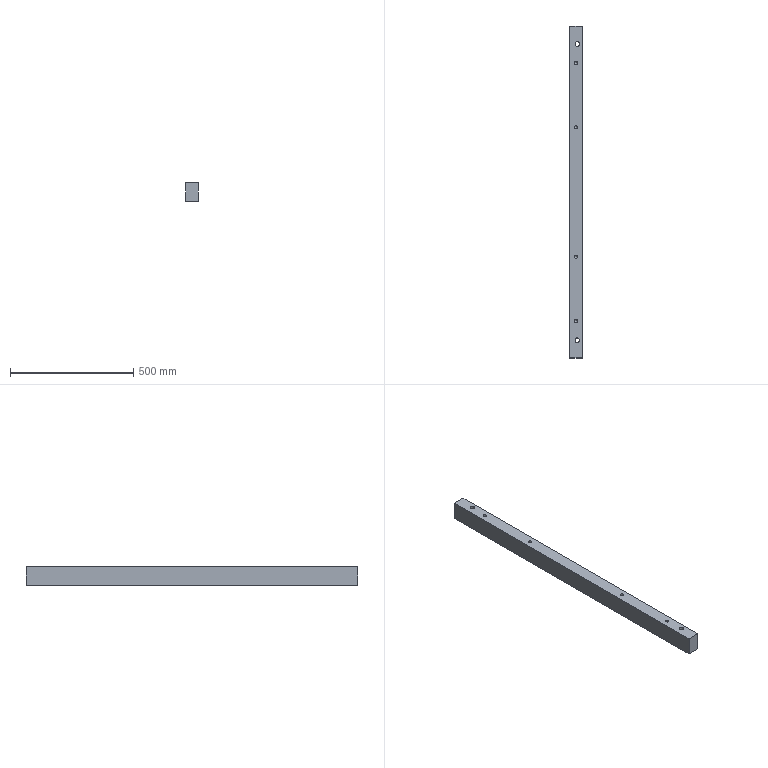Part | NX | features 3 2 | 1 solid | 24 faces | box 50 x 1345 x 75.5 mm | volume 5026084 mm3 | cylinder 10 | cone 8 | plane 6 | commonest cylinder face diameters 14.1 x8 18 x2
STEP:
#1=CARTESIAN_POINT('',(137.05,-262.5,256.5));
#2=VERTEX_POINT('',#1);
#3=CARTESIAN_POINT('',(130.,-262.5,256.5));
#4=DIRECTION('',(0.,0.,-1.));
#5=DIRECTION('',(1.,0.,0.));
#6=AXIS2_PLACEMENT_3D('',#3,#4,#5);
#7=CIRCLE('',#6,7.05);
#8=EDGE_CURVE('',#2,#2,#7,.T.);
#9=ORIENTED_EDGE('',*,*,#8,.T.);
#10=EDGE_LOOP('',(#9));
#11=FACE_BOUND('',#10,.T.);
#12=CARTESIAN_POINT('',(137.05,-522.5,256.5));
#13=VERTEX_POINT('',#12);
#14=CARTESIAN_POINT('',(130.,-522.5,256.5));
#15=DIRECTION('',(0.,0.,-1.));
#16=DIRECTION('',(1.,0.,0.));
#17=AXIS2_PLACEMENT_3D('',#14,#15,#16);
#18=CIRCLE('',#17,7.05);
#19=EDGE_CURVE('',#13,#13,#18,.T.);
#20=ORIENTED_EDGE('',*,*,#19,.T.);
#21=EDGE_LOOP('',(#20));
#22=FACE_BOUND('',#21,.T.);
#23=CARTESIAN_POINT('',(144.,-600.5,256.5));
#24=VERTEX_POINT('',#23);
#25=CARTESIAN_POINT('',(135.,-600.5,256.5));
#26=DIRECTION('',(0.,0.,-1.));
#27=DIRECTION('',(1.,0.,0.));
#28=AXIS2_PLACEMENT_3D('',#25,#26,#27);
#29=CIRCLE('',#28,9.);
#30=EDGE_CURVE('',#24,#24,#29,.T.);
#31=ORIENTED_EDGE('',*,*,#30,.T.);
#32=EDGE_LOOP('',(#31));
#33=FACE_BOUND('',#32,.T.);
#34=CARTESIAN_POINT('',(155.,-672.5,256.5));
#35=VERTEX_POINT('',#34);
#36=CARTESIAN_POINT('',(105.,-672.5,256.5));
#37=VERTEX_POINT('',#36);
#38=CARTESIAN_POINT('',(282.5,-672.5,256.5));
#39=DIRECTION('',(-1.,0.,0.));
#40=VECTOR('',#39,1000.);
#41=LINE('',#38,#40);
#42=EDGE_CURVE('',#35,#37,#41,.T.);
#43=ORIENTED_EDGE('',*,*,#42,.F.);
#44=CARTESIAN_POINT('',(155.,672.5,256.5));
#45=VERTEX_POINT('',#44);
#46=CARTESIAN_POINT('',(155.,193.,256.5));
#47=DIRECTION('',(0.,-1.,0.));
#48=VECTOR('',#47,1000.);
#49=LINE('',#46,#48);
#50=EDGE_CURVE('',#45,#35,#49,.T.);
#51=ORIENTED_EDGE('',*,*,#50,.F.);
#52=CARTESIAN_POINT('',(105.,672.5,256.5));
#53=VERTEX_POINT('',#52);
#54=CARTESIAN_POINT('',(105.,672.5,256.5));
#55=DIRECTION('',(1.,0.,0.));
#56=VECTOR('',#55,1000.);
#57=LINE('',#54,#56);
#58=EDGE_CURVE('',#53,#45,#57,.T.);
#59=ORIENTED_EDGE('',*,*,#58,.F.);
#60=CARTESIAN_POINT('',(105.,193.,256.5));
#61=DIRECTION('',(0.,1.,0.));
#62=VECTOR('',#61,1000.);
#63=LINE('',#60,#62);
#64=EDGE_CURVE('',#37,#53,#63,.T.);
#65=ORIENTED_EDGE('',*,*,#64,.F.);
#66=EDGE_LOOP('',(#43,#51,#59,#65));
#67=FACE_BOUND('',#66,.T.);
#68=CARTESIAN_POINT('',(144.,599.5,256.5));
#69=VERTEX_POINT('',#68);
#70=CARTESIAN_POINT('',(135.,599.5,256.5));
#71=DIRECTION('',(0.,0.,-1.));
#72=DIRECTION('',(1.,0.,0.));
#73=AXIS2_PLACEMENT_3D('',#70,#71,#72);
#74=CIRCLE('',#73,9.);
#75=EDGE_CURVE('',#69,#69,#74,.T.);
#76=ORIENTED_EDGE('',*,*,#75,.T.);
#77=EDGE_LOOP('',(#76));
#78=FACE_BOUND('',#77,.T.);
#79=CARTESIAN_POINT('',(137.05,262.5,256.5));
#80=VERTEX_POINT('',#79);
#81=CARTESIAN_POINT('',(130.,262.5,256.5));
#82=DIRECTION('',(0.,0.,-1.));
#83=DIRECTION('',(1.,0.,0.));
#84=AXIS2_PLACEMENT_3D('',#81,#82,#83);
#85=CIRCLE('',#84,7.05);
#86=EDGE_CURVE('',#80,#80,#85,.T.);
#87=ORIENTED_EDGE('',*,*,#86,.T.);
#88=EDGE_LOOP('',(#87));
#89=FACE_BOUND('',#88,.T.);
#90=CARTESIAN_POINT('',(137.05,522.5,256.5));
#91=VERTEX_POINT('',#90);
#92=CARTESIAN_POINT('',(130.,522.5,256.5));
#93=DIRECTION('',(0.,0.,-1.));
#94=DIRECTION('',(1.,0.,0.));
#95=AXIS2_PLACEMENT_3D('',#92,#93,#94);
#96=CIRCLE('',#95,7.05);
#97=EDGE_CURVE('',#91,#91,#96,.T.);
#98=ORIENTED_EDGE('',*,*,#97,.T.);
#99=EDGE_LOOP('',(#98));
#100=FACE_BOUND('',#99,.T.);
#101=CARTESIAN_POINT('',(2145.,0.,256.5));
#102=DIRECTION('',(0.,0.,1.));
#103=DIRECTION('',(-1.,0.,0.));
#104=AXIS2_PLACEMENT_3D('',#101,#102,#103);
#105=PLANE('',#104);
#106=ADVANCED_FACE('',(#11,#22,#33,#67,#78,#89,#100),#105,.T.);
#107=CARTESIAN_POINT('',(137.05,-262.5,181.));
#108=VERTEX_POINT('',#107);
#109=CARTESIAN_POINT('',(130.,-262.5,181.));
#110=DIRECTION('',(0.,0.,1.));
#111=DIRECTION('',(1.,0.,0.));
#112=AXIS2_PLACEMENT_3D('',#109,#110,#111);
#113=CIRCLE('',#112,7.05);
#114=EDGE_CURVE('',#108,#108,#113,.T.);
#115=ORIENTED_EDGE('',*,*,#114,.T.);
#116=EDGE_LOOP('',(#115));
#117=FACE_BOUND('',#116,.T.);
#118=CARTESIAN_POINT('',(137.05,262.5,181.));
#119=VERTEX_POINT('',#118);
#120=CARTESIAN_POINT('',(130.,262.5,181.));
#121=DIRECTION('',(0.,0.,1.));
#122=DIRECTION('',(1.,0.,0.));
#123=AXIS2_PLACEMENT_3D('',#120,#121,#122);
#124=CIRCLE('',#123,7.05);
#125=EDGE_CURVE('',#119,#119,#124,.T.);
#126=ORIENTED_EDGE('',*,*,#125,.T.);
#127=EDGE_LOOP('',(#126));
#128=FACE_BOUND('',#127,.T.);
#129=CARTESIAN_POINT('',(126.,-600.5,181.));
#130=VERTEX_POINT('',#129);
#131=CARTESIAN_POINT('',(135.,-600.5,181.));
#132=DIRECTION('',(0.,0.,1.));
#133=DIRECTION('',(-1.,0.,0.));
#134=AXIS2_PLACEMENT_3D('',#131,#132,#133);
#135=CIRCLE('',#134,9.);
#136=EDGE_CURVE('',#130,#130,#135,.T.);
#137=ORIENTED_EDGE('',*,*,#136,.T.);
#138=EDGE_LOOP('',(#137));
#139=FACE_BOUND('',#138,.T.);
#140=CARTESIAN_POINT('',(105.,672.5,181.));
#141=VERTEX_POINT('',#140);
#142=CARTESIAN_POINT('',(105.,-672.5,181.));
#143=VERTEX_POINT('',#142);
#144=CARTESIAN_POINT('',(105.,193.,181.));
#145=DIRECTION('',(0.,-1.,0.));
#146=VECTOR('',#145,1000.);
#147=LINE('',#144,#146);
#148=EDGE_CURVE('',#141,#143,#147,.T.);
#149=ORIENTED_EDGE('',*,*,#148,.F.);
#150=CARTESIAN_POINT('',(155.,672.5,181.));
#151=VERTEX_POINT('',#150);
#152=CARTESIAN_POINT('',(1375.,672.5,181.));
#153=DIRECTION('',(1.,0.,0.));
#154=VECTOR('',#153,1000.);
#155=LINE('',#152,#154);
#156=EDGE_CURVE('',#141,#151,#155,.T.);
#157=ORIENTED_EDGE('',*,*,#156,.T.);
#158=CARTESIAN_POINT('',(155.,-672.5,181.));
#159=VERTEX_POINT('',#158);
#160=CARTESIAN_POINT('',(155.,193.,181.));
#161=DIRECTION('',(0.,1.,0.));
#162=VECTOR('',#161,1000.);
#163=LINE('',#160,#162);
#164=EDGE_CURVE('',#159,#151,#163,.T.);
#165=ORIENTED_EDGE('',*,*,#164,.F.);
#166=CARTESIAN_POINT('',(1375.,-672.5,181.));
#167=DIRECTION('',(-1.,0.,0.));
#168=VECTOR('',#167,1000.);
#169=LINE('',#166,#168);
#170=EDGE_CURVE('',#159,#143,#169,.T.);
#171=ORIENTED_EDGE('',*,*,#170,.T.);
#172=EDGE_LOOP('',(#149,#157,#165,#171));
#173=FACE_BOUND('',#172,.T.);
#174=CARTESIAN_POINT('',(126.,599.5,181.));
#175=VERTEX_POINT('',#174);
#176=CARTESIAN_POINT('',(135.,599.5,181.));
#177=DIRECTION('',(0.,0.,-1.));
#178=DIRECTION('',(-1.,0.,0.));
#179=AXIS2_PLACEMENT_3D('',#176,#177,#178);
#180=CIRCLE('',#179,9.);
#181=EDGE_CURVE('',#175,#175,#180,.T.);
#182=ORIENTED_EDGE('',*,*,#181,.F.);
#183=EDGE_LOOP('',(#182));
#184=FACE_BOUND('',#183,.T.);
#185=CARTESIAN_POINT('',(137.05,-522.5,181.));
#186=VERTEX_POINT('',#185);
#187=CARTESIAN_POINT('',(130.,-522.5,181.));
#188=DIRECTION('',(0.,0.,1.));
#189=DIRECTION('',(1.,0.,0.));
#190=AXIS2_PLACEMENT_3D('',#187,#188,#189);
#191=CIRCLE('',#190,7.05);
#192=EDGE_CURVE('',#186,#186,#191,.T.);
#193=ORIENTED_EDGE('',*,*,#192,.T.);
#194=EDGE_LOOP('',(#193));
#195=FACE_BOUND('',#194,.T.);
#196=CARTESIAN_POINT('',(137.05,522.5,181.));
#197=VERTEX_POINT('',#196);
#198=CARTESIAN_POINT('',(130.,522.5,181.));
#199=DIRECTION('',(0.,0.,1.));
#200=DIRECTION('',(1.,0.,0.));
#201=AXIS2_PLACEMENT_3D('',#198,#199,#200);
#202=CIRCLE('',#201,7.05);
#203=EDGE_CURVE('',#197,#197,#202,.T.);
#204=ORIENTED_EDGE('',*,*,#203,.T.);
#205=EDGE_LOOP('',(#204));
#206=FACE_BOUND('',#205,.T.);
#207=CARTESIAN_POINT('',(1375.,193.,181.));
#208=DIRECTION('',(0.,0.,-1.));
#209=DIRECTION('',(-1.,0.,0.));
#210=AXIS2_PLACEMENT_3D('',#207,#208,#209);
#211=PLANE('',#210);
#212=ADVANCED_FACE('',(#117,#128,#139,#173,#184,#195,#206),#211,.T.);
#213=CARTESIAN_POINT('',(105.,-672.5,-1.5));
#214=DIRECTION('',(0.,0.,1.));
#215=VECTOR('',#214,1000.);
#216=LINE('',#213,#215);
#217=EDGE_CURVE('',#143,#37,#216,.T.);
#218=ORIENTED_EDGE('',*,*,#217,.T.);
#219=ORIENTED_EDGE('',*,*,#64,.T.);
#220=CARTESIAN_POINT('',(105.,672.5,-1.5));
#221=DIRECTION('',(0.,0.,-1.));
#222=VECTOR('',#221,1000.);
#223=LINE('',#220,#222);
#224=EDGE_CURVE('',#53,#141,#223,.T.);
#225=ORIENTED_EDGE('',*,*,#224,.T.);
#226=ORIENTED_EDGE('',*,*,#148,.T.);
#227=EDGE_LOOP('',(#218,#219,#225,#226));
#228=FACE_BOUND('',#227,.T.);
#229=CARTESIAN_POINT('',(105.,193.,-1.5));
#230=DIRECTION('',(-1.,0.,0.));
#231=DIRECTION('',(0.,0.,-1.));
#232=AXIS2_PLACEMENT_3D('',#229,#230,#231);
#233=PLANE('',#232);
#234=ADVANCED_FACE('',(#228),#233,.T.);
#235=CARTESIAN_POINT('',(155.,672.5,-1.5));
#236=DIRECTION('',(0.,0.,1.));
#237=VECTOR('',#236,1000.);
#238=LINE('',#235,#237);
#239=EDGE_CURVE('',#151,#45,#238,.T.);
#240=ORIENTED_EDGE('',*,*,#239,.T.);
#241=ORIENTED_EDGE('',*,*,#50,.T.);
#242=CARTESIAN_POINT('',(155.,-672.5,-1.5));
#243=DIRECTION('',(0.,0.,-1.));
#244=VECTOR('',#243,1000.);
#245=LINE('',#242,#244);
#246=EDGE_CURVE('',#35,#159,#245,.T.);
#247=ORIENTED_EDGE('',*,*,#246,.T.);
#248=ORIENTED_EDGE('',*,*,#164,.T.);
#249=EDGE_LOOP('',(#240,#241,#247,#248));
#250=FACE_BOUND('',#249,.T.);
#251=CARTESIAN_POINT('',(155.,193.,-1.5));
#252=DIRECTION('',(1.,0.,0.));
#253=DIRECTION('',(0.,0.,1.));
#254=AXIS2_PLACEMENT_3D('',#251,#252,#253);
#255=PLANE('',#254);
#256=ADVANCED_FACE('',(#250),#255,.T.);
#257=ORIENTED_EDGE('',*,*,#246,.F.);
#258=ORIENTED_EDGE('',*,*,#42,.T.);
#259=ORIENTED_EDGE('',*,*,#217,.F.);
#260=ORIENTED_EDGE('',*,*,#170,.F.);
#261=EDGE_LOOP('',(#257,#258,#259,#260));
#262=FACE_BOUND('',#261,.T.);
#263=CARTESIAN_POINT('',(282.5,-672.5,-103.));
#264=DIRECTION('',(0.,1.,0.));
#265=DIRECTION('',(1.,0.,0.));
#266=AXIS2_PLACEMENT_3D('',#263,#264,#265);
#267=PLANE('',#266);
#268=ADVANCED_FACE('',(#262),#267,.F.);
#269=ORIENTED_EDGE('',*,*,#224,.F.);
#270=ORIENTED_EDGE('',*,*,#58,.T.);
#271=ORIENTED_EDGE('',*,*,#239,.F.);
#272=ORIENTED_EDGE('',*,*,#156,.F.);
#273=EDGE_LOOP('',(#269,#270,#271,#272));
#274=FACE_BOUND('',#273,.T.);
#275=CARTESIAN_POINT('',(105.,672.5,231.5));
#276=DIRECTION('',(0.,1.,0.));
#277=DIRECTION('',(0.,0.,-1.));
#278=AXIS2_PLACEMENT_3D('',#275,#276,#277);
#279=PLANE('',#278);
#280=ADVANCED_FACE('',(#274),#279,.T.);
#281=ORIENTED_EDGE('',*,*,#30,.F.);
#282=EDGE_LOOP('',(#281));
#283=FACE_BOUND('',#282,.T.);
#284=ORIENTED_EDGE('',*,*,#136,.F.);
#285=EDGE_LOOP('',(#284));
#286=FACE_BOUND('',#285,.T.);
#287=CARTESIAN_POINT('',(135.,-600.5,-306.5));
#288=DIRECTION('',(0.,0.,1.));
#289=DIRECTION('',(-1.,0.,0.));
#290=AXIS2_PLACEMENT_3D('',#287,#288,#289);
#291=CYLINDRICAL_SURFACE('',#290,9.);
#292=ADVANCED_FACE('',(#283,#286),#291,.F.);
#293=ORIENTED_EDGE('',*,*,#75,.F.);
#294=EDGE_LOOP('',(#293));
#295=FACE_BOUND('',#294,.T.);
#296=ORIENTED_EDGE('',*,*,#181,.T.);
#297=EDGE_LOOP('',(#296));
#298=FACE_BOUND('',#297,.T.);
#299=CARTESIAN_POINT('',(135.,599.5,-306.5));
#300=DIRECTION('',(0.,0.,1.));
#301=DIRECTION('',(-1.,0.,0.));
#302=AXIS2_PLACEMENT_3D('',#299,#300,#301);
#303=CYLINDRICAL_SURFACE('',#302,9.);
#304=ADVANCED_FACE('',(#295,#298),#303,.F.);
#305=ORIENTED_EDGE('',*,*,#125,.F.);
#306=EDGE_LOOP('',(#305));
#307=FACE_BOUND('',#306,.T.);
#308=CARTESIAN_POINT('',(137.05,262.5,188.95));
#309=VERTEX_POINT('',#308);
#310=CARTESIAN_POINT('',(130.,262.5,188.95));
#311=DIRECTION('',(0.,0.,-1.));
#312=DIRECTION('',(1.,0.,0.));
#313=AXIS2_PLACEMENT_3D('',#310,#311,#312);
#314=CIRCLE('',#313,7.05);
#315=EDGE_CURVE('',#309,#309,#314,.T.);
#316=ORIENTED_EDGE('',*,*,#315,.F.);
#317=EDGE_LOOP('',(#316));
#318=FACE_BOUND('',#317,.T.);
#319=CARTESIAN_POINT('',(130.,262.5,181.));
#320=DIRECTION('',(0.,0.,1.));
#321=DIRECTION('',(-1.,0.,0.));
#322=AXIS2_PLACEMENT_3D('',#319,#320,#321);
#323=CYLINDRICAL_SURFACE('',#322,7.05);
#324=ADVANCED_FACE('',(#307,#318),#323,.F.);
#325=ORIENTED_EDGE('',*,*,#192,.F.);
#326=EDGE_LOOP('',(#325));
#327=FACE_BOUND('',#326,.T.);
#328=CARTESIAN_POINT('',(137.05,-522.5,188.95));
#329=VERTEX_POINT('',#328);
#330=CARTESIAN_POINT('',(130.,-522.5,188.95));
#331=DIRECTION('',(0.,0.,-1.));
#332=DIRECTION('',(1.,0.,0.));
#333=AXIS2_PLACEMENT_3D('',#330,#331,#332);
#334=CIRCLE('',#333,7.05);
#335=EDGE_CURVE('',#329,#329,#334,.T.);
#336=ORIENTED_EDGE('',*,*,#335,.F.);
#337=EDGE_LOOP('',(#336));
#338=FACE_BOUND('',#337,.T.);
#339=CARTESIAN_POINT('',(130.,-522.5,181.));
#340=DIRECTION('',(0.,0.,1.));
#341=DIRECTION('',(-1.,0.,0.));
#342=AXIS2_PLACEMENT_3D('',#339,#340,#341);
#343=CYLINDRICAL_SURFACE('',#342,7.05);
#344=ADVANCED_FACE('',(#327,#338),#343,.F.);
#345=ORIENTED_EDGE('',*,*,#114,.F.);
#346=EDGE_LOOP('',(#345));
#347=FACE_BOUND('',#346,.T.);
#348=CARTESIAN_POINT('',(137.05,-262.5,188.95));
#349=VERTEX_POINT('',#348);
#350=CARTESIAN_POINT('',(130.,-262.5,188.95));
#351=DIRECTION('',(0.,0.,-1.));
#352=DIRECTION('',(1.,0.,0.));
#353=AXIS2_PLACEMENT_3D('',#350,#351,#352);
#354=CIRCLE('',#353,7.05);
#355=EDGE_CURVE('',#349,#349,#354,.T.);
#356=ORIENTED_EDGE('',*,*,#355,.F.);
#357=EDGE_LOOP('',(#356));
#358=FACE_BOUND('',#357,.T.);
#359=CARTESIAN_POINT('',(130.,-262.5,181.));
#360=DIRECTION('',(0.,0.,1.));
#361=DIRECTION('',(-1.,0.,0.));
#362=AXIS2_PLACEMENT_3D('',#359,#360,#361);
#363=CYLINDRICAL_SURFACE('',#362,7.05);
#364=ADVANCED_FACE('',(#347,#358),#363,.F.);
#365=ORIENTED_EDGE('',*,*,#203,.F.);
#366=EDGE_LOOP('',(#365));
#367=FACE_BOUND('',#366,.T.);
#368=CARTESIAN_POINT('',(137.05,522.5,188.95));
#369=VERTEX_POINT('',#368);
#370=CARTESIAN_POINT('',(130.,522.5,188.95));
#371=DIRECTION('',(0.,0.,-1.));
#372=DIRECTION('',(1.,0.,0.));
#373=AXIS2_PLACEMENT_3D('',#370,#371,#372);
#374=CIRCLE('',#373,7.05);
#375=EDGE_CURVE('',#369,#369,#374,.T.);
#376=ORIENTED_EDGE('',*,*,#375,.F.);
#377=EDGE_LOOP('',(#376));
#378=FACE_BOUND('',#377,.T.);
#379=CARTESIAN_POINT('',(130.,522.5,181.));
#380=DIRECTION('',(0.,0.,1.));
#381=DIRECTION('',(-1.,0.,0.));
#382=AXIS2_PLACEMENT_3D('',#379,#380,#381);
#383=CYLINDRICAL_SURFACE('',#382,7.05);
#384=ADVANCED_FACE('',(#367,#378),#383,.F.);
#385=CARTESIAN_POINT('',(130.,262.5,196.));
#386=VERTEX_POINT('',#385);
#387=VERTEX_LOOP('',#386);
#388=FACE_BOUND('',#387,.T.);
#389=ORIENTED_EDGE('',*,*,#315,.T.);
#390=EDGE_LOOP('',(#389));
#391=FACE_BOUND('',#390,.T.);
#392=CARTESIAN_POINT('',(130.,262.5,188.95));
#393=DIRECTION('',(0.,0.,-1.));
#394=DIRECTION('',(1.,0.,0.));
#395=AXIS2_PLACEMENT_3D('',#392,#393,#394);
#396=CONICAL_SURFACE('',#395,7.05,0.7854);
#397=ADVANCED_FACE('',(#388,#391),#396,.F.);
#398=CARTESIAN_POINT('',(130.,-522.5,196.));
#399=VERTEX_POINT('',#398);
#400=VERTEX_LOOP('',#399);
#401=FACE_BOUND('',#400,.T.);
#402=ORIENTED_EDGE('',*,*,#335,.T.);
#403=EDGE_LOOP('',(#402));
#404=FACE_BOUND('',#403,.T.);
#405=CARTESIAN_POINT('',(130.,-522.5,188.95));
#406=DIRECTION('',(0.,0.,-1.));
#407=DIRECTION('',(1.,0.,0.));
#408=AXIS2_PLACEMENT_3D('',#405,#406,#407);
#409=CONICAL_SURFACE('',#408,7.05,0.7854);
#410=ADVANCED_FACE('',(#401,#404),#409,.F.);
#411=CARTESIAN_POINT('',(130.,-262.5,196.));
#412=VERTEX_POINT('',#411);
#413=VERTEX_LOOP('',#412);
#414=FACE_BOUND('',#413,.T.);
#415=ORIENTED_EDGE('',*,*,#355,.T.);
#416=EDGE_LOOP('',(#415));
#417=FACE_BOUND('',#416,.T.);
#418=CARTESIAN_POINT('',(130.,-262.5,188.95));
#419=DIRECTION('',(0.,0.,-1.));
#420=DIRECTION('',(1.,0.,0.));
#421=AXIS2_PLACEMENT_3D('',#418,#419,#420);
#422=CONICAL_SURFACE('',#421,7.05,0.7854);
#423=ADVANCED_FACE('',(#414,#417),#422,.F.);
#424=CARTESIAN_POINT('',(130.,522.5,196.));
#425=VERTEX_POINT('',#424);
#426=VERTEX_LOOP('',#425);
#427=FACE_BOUND('',#426,.T.);
#428=ORIENTED_EDGE('',*,*,#375,.T.);
#429=EDGE_LOOP('',(#428));
#430=FACE_BOUND('',#429,.T.);
#431=CARTESIAN_POINT('',(130.,522.5,188.95));
#432=DIRECTION('',(0.,0.,-1.));
#433=DIRECTION('',(1.,0.,0.));
#434=AXIS2_PLACEMENT_3D('',#431,#432,#433);
#435=CONICAL_SURFACE('',#434,7.05,0.7854);
#436=ADVANCED_FACE('',(#427,#430),#435,.F.);
#437=CARTESIAN_POINT('',(122.95,-522.5,248.55));
#438=VERTEX_POINT('',#437);
#439=CARTESIAN_POINT('',(130.,-522.5,248.55));
#440=DIRECTION('',(0.,0.,-1.));
#441=DIRECTION('',(-1.,0.,0.));
#442=AXIS2_PLACEMENT_3D('',#439,#440,#441);
#443=CIRCLE('',#442,7.05);
#444=EDGE_CURVE('',#438,#438,#443,.T.);
#445=ORIENTED_EDGE('',*,*,#444,.T.);
#446=EDGE_LOOP('',(#445));
#447=FACE_BOUND('',#446,.T.);
#448=ORIENTED_EDGE('',*,*,#19,.F.);
#449=EDGE_LOOP('',(#448));
#450=FACE_BOUND('',#449,.T.);
#451=CARTESIAN_POINT('',(130.,-522.5,256.5));
#452=DIRECTION('',(0.,0.,-1.));
#453=DIRECTION('',(-1.,0.,0.));
#454=AXIS2_PLACEMENT_3D('',#451,#452,#453);
#455=CYLINDRICAL_SURFACE('',#454,7.05);
#456=ADVANCED_FACE('',(#447,#450),#455,.F.);
#457=CARTESIAN_POINT('',(130.,-522.5,241.5));
#458=VERTEX_POINT('',#457);
#459=VERTEX_LOOP('',#458);
#460=FACE_BOUND('',#459,.T.);
#461=ORIENTED_EDGE('',*,*,#444,.F.);
#462=EDGE_LOOP('',(#461));
#463=FACE_BOUND('',#462,.T.);
#464=CARTESIAN_POINT('',(130.,-522.5,248.55));
#465=DIRECTION('',(0.,0.,1.));
#466=DIRECTION('',(-1.,0.,0.));
#467=AXIS2_PLACEMENT_3D('',#464,#465,#466);
#468=CONICAL_SURFACE('',#467,7.05,0.7854);
#469=ADVANCED_FACE('',(#460,#463),#468,.F.);
#470=CARTESIAN_POINT('',(122.95,262.5,248.55));
#471=VERTEX_POINT('',#470);
#472=CARTESIAN_POINT('',(130.,262.5,248.55));
#473=DIRECTION('',(0.,0.,-1.));
#474=DIRECTION('',(-1.,0.,0.));
#475=AXIS2_PLACEMENT_3D('',#472,#473,#474);
#476=CIRCLE('',#475,7.05);
#477=EDGE_CURVE('',#471,#471,#476,.T.);
#478=ORIENTED_EDGE('',*,*,#477,.T.);
#479=EDGE_LOOP('',(#478));
#480=FACE_BOUND('',#479,.T.);
#481=ORIENTED_EDGE('',*,*,#86,.F.);
#482=EDGE_LOOP('',(#481));
#483=FACE_BOUND('',#482,.T.);
#484=CARTESIAN_POINT('',(130.,262.5,256.5));
#485=DIRECTION('',(0.,0.,-1.));
#486=DIRECTION('',(-1.,0.,0.));
#487=AXIS2_PLACEMENT_3D('',#484,#485,#486);
#488=CYLINDRICAL_SURFACE('',#487,7.05);
#489=ADVANCED_FACE('',(#480,#483),#488,.F.);
#490=CARTESIAN_POINT('',(130.,262.5,241.5));
#491=VERTEX_POINT('',#490);
#492=VERTEX_LOOP('',#491);
#493=FACE_BOUND('',#492,.T.);
#494=ORIENTED_EDGE('',*,*,#477,.F.);
#495=EDGE_LOOP('',(#494));
#496=FACE_BOUND('',#495,.T.);
#497=CARTESIAN_POINT('',(130.,262.5,248.55));
#498=DIRECTION('',(0.,0.,1.));
#499=DIRECTION('',(-1.,0.,0.));
#500=AXIS2_PLACEMENT_3D('',#497,#498,#499);
#501=CONICAL_SURFACE('',#500,7.05,0.7854);
#502=ADVANCED_FACE('',(#493,#496),#501,.F.);
#503=CARTESIAN_POINT('',(122.95,-262.5,248.55));
#504=VERTEX_POINT('',#503);
#505=CARTESIAN_POINT('',(130.,-262.5,248.55));
#506=DIRECTION('',(0.,0.,-1.));
#507=DIRECTION('',(-1.,0.,0.));
#508=AXIS2_PLACEMENT_3D('',#505,#506,#507);
#509=CIRCLE('',#508,7.05);
#510=EDGE_CURVE('',#504,#504,#509,.T.);
#511=ORIENTED_EDGE('',*,*,#510,.T.);
#512=EDGE_LOOP('',(#511));
#513=FACE_BOUND('',#512,.T.);
#514=ORIENTED_EDGE('',*,*,#8,.F.);
#515=EDGE_LOOP('',(#514));
#516=FACE_BOUND('',#515,.T.);
#517=CARTESIAN_POINT('',(130.,-262.5,256.5));
#518=DIRECTION('',(0.,0.,-1.));
#519=DIRECTION('',(-1.,0.,0.));
#520=AXIS2_PLACEMENT_3D('',#517,#518,#519);
#521=CYLINDRICAL_SURFACE('',#520,7.05);
#522=ADVANCED_FACE('',(#513,#516),#521,.F.);
#523=CARTESIAN_POINT('',(130.,-262.5,241.5));
#524=VERTEX_POINT('',#523);
#525=VERTEX_LOOP('',#524);
#526=FACE_BOUND('',#525,.T.);
#527=ORIENTED_EDGE('',*,*,#510,.F.);
#528=EDGE_LOOP('',(#527));
#529=FACE_BOUND('',#528,.T.);
#530=CARTESIAN_POINT('',(130.,-262.5,248.55));
#531=DIRECTION('',(0.,0.,1.));
#532=DIRECTION('',(-1.,0.,0.));
#533=AXIS2_PLACEMENT_3D('',#530,#531,#532);
#534=CONICAL_SURFACE('',#533,7.05,0.7854);
#535=ADVANCED_FACE('',(#526,#529),#534,.F.);
#536=CARTESIAN_POINT('',(122.95,522.5,248.55));
#537=VERTEX_POINT('',#536);
#538=CARTESIAN_POINT('',(130.,522.5,248.55));
#539=DIRECTION('',(0.,0.,-1.));
#540=DIRECTION('',(-1.,0.,0.));
#541=AXIS2_PLACEMENT_3D('',#538,#539,#540);
#542=CIRCLE('',#541,7.05);
#543=EDGE_CURVE('',#537,#537,#542,.T.);
#544=ORIENTED_EDGE('',*,*,#543,.T.);
#545=EDGE_LOOP('',(#544));
#546=FACE_BOUND('',#545,.T.);
#547=ORIENTED_EDGE('',*,*,#97,.F.);
#548=EDGE_LOOP('',(#547));
#549=FACE_BOUND('',#548,.T.);
#550=CARTESIAN_POINT('',(130.,522.5,256.5));
#551=DIRECTION('',(0.,0.,-1.));
#552=DIRECTION('',(-1.,0.,0.));
#553=AXIS2_PLACEMENT_3D('',#550,#551,#552);
#554=CYLINDRICAL_SURFACE('',#553,7.05);
#555=ADVANCED_FACE('',(#546,#549),#554,.F.);
#556=CARTESIAN_POINT('',(130.,522.5,241.5));
#557=VERTEX_POINT('',#556);
#558=VERTEX_LOOP('',#557);
#559=FACE_BOUND('',#558,.T.);
#560=ORIENTED_EDGE('',*,*,#543,.F.);
#561=EDGE_LOOP('',(#560));
#562=FACE_BOUND('',#561,.T.);
#563=CARTESIAN_POINT('',(130.,522.5,248.55));
#564=DIRECTION('',(0.,0.,1.));
#565=DIRECTION('',(-1.,0.,0.));
#566=AXIS2_PLACEMENT_3D('',#563,#564,#565);
#567=CONICAL_SURFACE('',#566,7.05,0.7854);
#568=ADVANCED_FACE('',(#559,#562),#567,.F.);
#569=CLOSED_SHELL('',(#106,#212,#234,#256,#268,#280,#292,#304,#324,#344,#364,#384,#397,#410,#423,#436,#456,#469,#489,#502,#522,#535,#555,#568));
#570=MANIFOLD_SOLID_BREP('',#569);
#571=(LENGTH_UNIT()NAMED_UNIT(*)SI_UNIT(.MILLI.,.METRE.));
#572=UNCERTAINTY_MEASURE_WITH_UNIT(LENGTH_MEASURE(0.00001),#571,'','');
#573=(NAMED_UNIT(*)PLANE_ANGLE_UNIT()SI_UNIT($,.RADIAN.));
#574=(NAMED_UNIT(*)SI_UNIT($,.STERADIAN.)SOLID_ANGLE_UNIT());
#575=(GEOMETRIC_REPRESENTATION_CONTEXT(3)GLOBAL_UNCERTAINTY_ASSIGNED_CONTEXT((#572))GLOBAL_UNIT_ASSIGNED_CONTEXT((#571,#573,#574))REPRESENTATION_CONTEXT('',''));
#576=ADVANCED_BREP_SHAPE_REPRESENTATION('',(#570),#575);